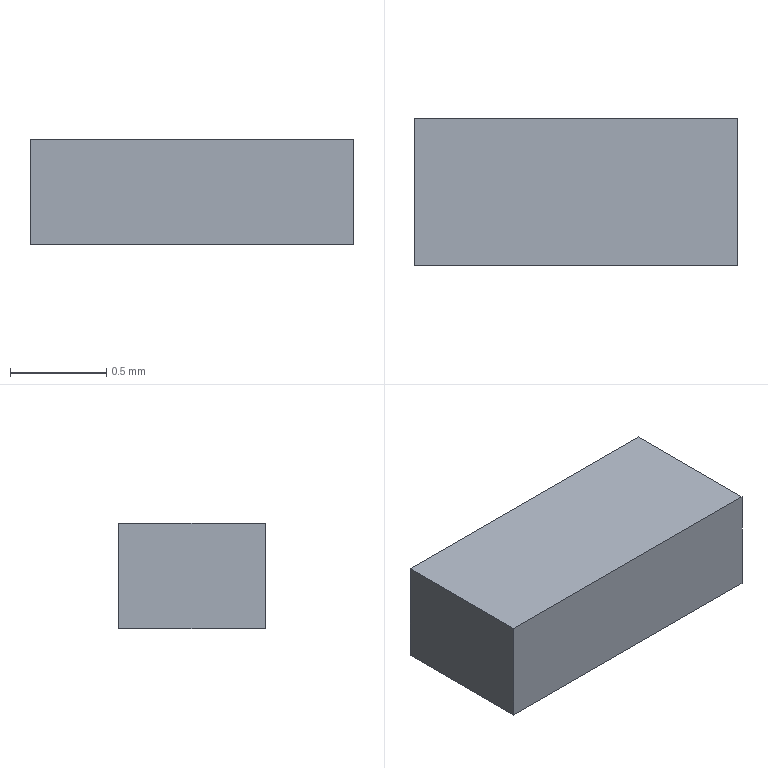Part | Creo | 1 solid | 6 faces | box 1.676 x 0.762 x 0.55 mm | volume 0.7026 mm3 | plane 6
STEP:
#1=CARTESIAN_POINT('',(0.,0.,0.));
#2=DIRECTION('',(0.,0.,1.));
#3=DIRECTION('',(1.,0.,0.));
#4=AXIS2_PLACEMENT_3D('',#1,#2,#3);
#5=CARTESIAN_POINT('',(0.8382,-0.381,0.));
#6=VERTEX_POINT('',#5);
#7=CARTESIAN_POINT('',(0.8382,0.381,0.));
#8=VERTEX_POINT('',#7);
#9=CARTESIAN_POINT('',(0.8382,-0.381,0.));
#10=DIRECTION('',(0.,1.,0.));
#11=VECTOR('',#10,0.762);
#12=LINE('',#9,#11);
#13=EDGE_CURVE('',#6,#8,#12,.T.);
#14=ORIENTED_EDGE('',*,*,#13,.T.);
#15=CARTESIAN_POINT('',(-0.8382,0.381,0.));
#16=VERTEX_POINT('',#15);
#17=CARTESIAN_POINT('',(0.8382,0.381,0.));
#18=DIRECTION('',(-1.,0.,0.));
#19=VECTOR('',#18,1.676);
#20=LINE('',#17,#19);
#21=EDGE_CURVE('',#8,#16,#20,.T.);
#22=ORIENTED_EDGE('',*,*,#21,.T.);
#23=CARTESIAN_POINT('',(-0.8382,-0.381,0.));
#24=VERTEX_POINT('',#23);
#25=CARTESIAN_POINT('',(-0.8382,0.381,0.));
#26=DIRECTION('',(0.,-1.,0.));
#27=VECTOR('',#26,0.762);
#28=LINE('',#25,#27);
#29=EDGE_CURVE('',#16,#24,#28,.T.);
#30=ORIENTED_EDGE('',*,*,#29,.T.);
#31=CARTESIAN_POINT('',(-0.8382,-0.381,0.));
#32=DIRECTION('',(1.,0.,0.));
#33=VECTOR('',#32,1.676);
#34=LINE('',#31,#33);
#35=EDGE_CURVE('',#24,#6,#34,.T.);
#36=ORIENTED_EDGE('',*,*,#35,.T.);
#37=EDGE_LOOP('',(#14,#22,#30,#36));
#38=FACE_OUTER_BOUND('',#37,.F.);
#39=CARTESIAN_POINT('',(0.,0.,0.));
#40=DIRECTION('',(0.,0.,1.));
#41=DIRECTION('',(1.,0.,0.));
#42=AXIS2_PLACEMENT_3D('',#39,#40,#41);
#43=PLANE('',#42);
#44=ADVANCED_FACE('',(#38),#43,.F.);
#45=ORIENTED_EDGE('',*,*,#13,.F.);
#46=CARTESIAN_POINT('',(0.8382,-0.381,0.55));
#47=VERTEX_POINT('',#46);
#48=CARTESIAN_POINT('',(0.8382,-0.381,0.));
#49=DIRECTION('',(0.,0.,1.));
#50=VECTOR('',#49,0.55);
#51=LINE('',#48,#50);
#52=EDGE_CURVE('',#6,#47,#51,.T.);
#53=ORIENTED_EDGE('',*,*,#52,.T.);
#54=CARTESIAN_POINT('',(0.8382,0.381,0.55));
#55=VERTEX_POINT('',#54);
#56=CARTESIAN_POINT('',(0.8382,-0.381,0.55));
#57=DIRECTION('',(0.,1.,0.));
#58=VECTOR('',#57,0.762);
#59=LINE('',#56,#58);
#60=EDGE_CURVE('',#47,#55,#59,.T.);
#61=ORIENTED_EDGE('',*,*,#60,.T.);
#62=CARTESIAN_POINT('',(0.8382,0.381,0.));
#63=DIRECTION('',(0.,0.,1.));
#64=VECTOR('',#63,0.55);
#65=LINE('',#62,#64);
#66=EDGE_CURVE('',#8,#55,#65,.T.);
#67=ORIENTED_EDGE('',*,*,#66,.F.);
#68=EDGE_LOOP('',(#45,#53,#61,#67));
#69=FACE_OUTER_BOUND('',#68,.F.);
#70=CARTESIAN_POINT('',(0.8382,-0.381,0.));
#71=DIRECTION('',(1.,0.,0.));
#72=DIRECTION('',(0.,1.,0.));
#73=AXIS2_PLACEMENT_3D('',#70,#71,#72);
#74=PLANE('',#73);
#75=ADVANCED_FACE('',(#69),#74,.T.);
#76=ORIENTED_EDGE('',*,*,#35,.F.);
#77=CARTESIAN_POINT('',(-0.8382,-0.381,0.55));
#78=VERTEX_POINT('',#77);
#79=CARTESIAN_POINT('',(-0.8382,-0.381,0.));
#80=DIRECTION('',(0.,0.,1.));
#81=VECTOR('',#80,0.55);
#82=LINE('',#79,#81);
#83=EDGE_CURVE('',#24,#78,#82,.T.);
#84=ORIENTED_EDGE('',*,*,#83,.T.);
#85=CARTESIAN_POINT('',(-0.8382,-0.381,0.55));
#86=DIRECTION('',(1.,0.,0.));
#87=VECTOR('',#86,1.676);
#88=LINE('',#85,#87);
#89=EDGE_CURVE('',#78,#47,#88,.T.);
#90=ORIENTED_EDGE('',*,*,#89,.T.);
#91=ORIENTED_EDGE('',*,*,#52,.F.);
#92=EDGE_LOOP('',(#76,#84,#90,#91));
#93=FACE_OUTER_BOUND('',#92,.F.);
#94=CARTESIAN_POINT('',(-0.8382,-0.381,0.));
#95=DIRECTION('',(0.,-1.,0.));
#96=DIRECTION('',(1.,0.,0.));
#97=AXIS2_PLACEMENT_3D('',#94,#95,#96);
#98=PLANE('',#97);
#99=ADVANCED_FACE('',(#93),#98,.T.);
#100=ORIENTED_EDGE('',*,*,#29,.F.);
#101=CARTESIAN_POINT('',(-0.8382,0.381,0.55));
#102=VERTEX_POINT('',#101);
#103=CARTESIAN_POINT('',(-0.8382,0.381,0.));
#104=DIRECTION('',(0.,0.,1.));
#105=VECTOR('',#104,0.55);
#106=LINE('',#103,#105);
#107=EDGE_CURVE('',#16,#102,#106,.T.);
#108=ORIENTED_EDGE('',*,*,#107,.T.);
#109=CARTESIAN_POINT('',(-0.8382,0.381,0.55));
#110=DIRECTION('',(0.,-1.,0.));
#111=VECTOR('',#110,0.762);
#112=LINE('',#109,#111);
#113=EDGE_CURVE('',#102,#78,#112,.T.);
#114=ORIENTED_EDGE('',*,*,#113,.T.);
#115=ORIENTED_EDGE('',*,*,#83,.F.);
#116=EDGE_LOOP('',(#100,#108,#114,#115));
#117=FACE_OUTER_BOUND('',#116,.F.);
#118=CARTESIAN_POINT('',(-0.8382,0.381,0.));
#119=DIRECTION('',(-1.,0.,0.));
#120=DIRECTION('',(0.,-1.,0.));
#121=AXIS2_PLACEMENT_3D('',#118,#119,#120);
#122=PLANE('',#121);
#123=ADVANCED_FACE('',(#117),#122,.T.);
#124=ORIENTED_EDGE('',*,*,#21,.F.);
#125=ORIENTED_EDGE('',*,*,#66,.T.);
#126=CARTESIAN_POINT('',(0.8382,0.381,0.55));
#127=DIRECTION('',(-1.,0.,0.));
#128=VECTOR('',#127,1.676);
#129=LINE('',#126,#128);
#130=EDGE_CURVE('',#55,#102,#129,.T.);
#131=ORIENTED_EDGE('',*,*,#130,.T.);
#132=ORIENTED_EDGE('',*,*,#107,.F.);
#133=EDGE_LOOP('',(#124,#125,#131,#132));
#134=FACE_OUTER_BOUND('',#133,.F.);
#135=CARTESIAN_POINT('',(0.8382,0.381,0.));
#136=DIRECTION('',(0.,1.,0.));
#137=DIRECTION('',(-1.,0.,0.));
#138=AXIS2_PLACEMENT_3D('',#135,#136,#137);
#139=PLANE('',#138);
#140=ADVANCED_FACE('',(#134),#139,.T.);
#141=ORIENTED_EDGE('',*,*,#60,.F.);
#142=ORIENTED_EDGE('',*,*,#89,.F.);
#143=ORIENTED_EDGE('',*,*,#113,.F.);
#144=ORIENTED_EDGE('',*,*,#130,.F.);
#145=EDGE_LOOP('',(#141,#142,#143,#144));
#146=FACE_OUTER_BOUND('',#145,.F.);
#147=CARTESIAN_POINT('',(0.,0.,0.55));
#148=DIRECTION('',(0.,0.,1.));
#149=DIRECTION('',(1.,0.,0.));
#150=AXIS2_PLACEMENT_3D('',#147,#148,#149);
#151=PLANE('',#150);
#152=ADVANCED_FACE('',(#146),#151,.T.);
#153=CLOSED_SHELL('',(#44,#75,#99,#123,#140,#152));
#154=MANIFOLD_SOLID_BREP('',#153);
#155=(LENGTH_UNIT()NAMED_UNIT(*)SI_UNIT(.MILLI.,.METRE.));
#156=UNCERTAINTY_MEASURE_WITH_UNIT(LENGTH_MEASURE(0.0001922),#155,'','');
#157=(NAMED_UNIT(*)PLANE_ANGLE_UNIT()SI_UNIT($,.RADIAN.));
#158=PLANE_ANGLE_MEASURE_WITH_UNIT(PLANE_ANGLE_MEASURE(0.01745),#157);
#159=(CONVERSION_BASED_UNIT('DEGREE',#158)NAMED_UNIT(*)PLANE_ANGLE_UNIT());
#160=(NAMED_UNIT(*)SI_UNIT($,.STERADIAN.)SOLID_ANGLE_UNIT());
#161=(GEOMETRIC_REPRESENTATION_CONTEXT(3)GLOBAL_UNCERTAINTY_ASSIGNED_CONTEXT((#156))GLOBAL_UNIT_ASSIGNED_CONTEXT((#155,#159,#160))REPRESENTATION_CONTEXT('',''));
#162=ADVANCED_BREP_SHAPE_REPRESENTATION('',(#4,#154),#161);